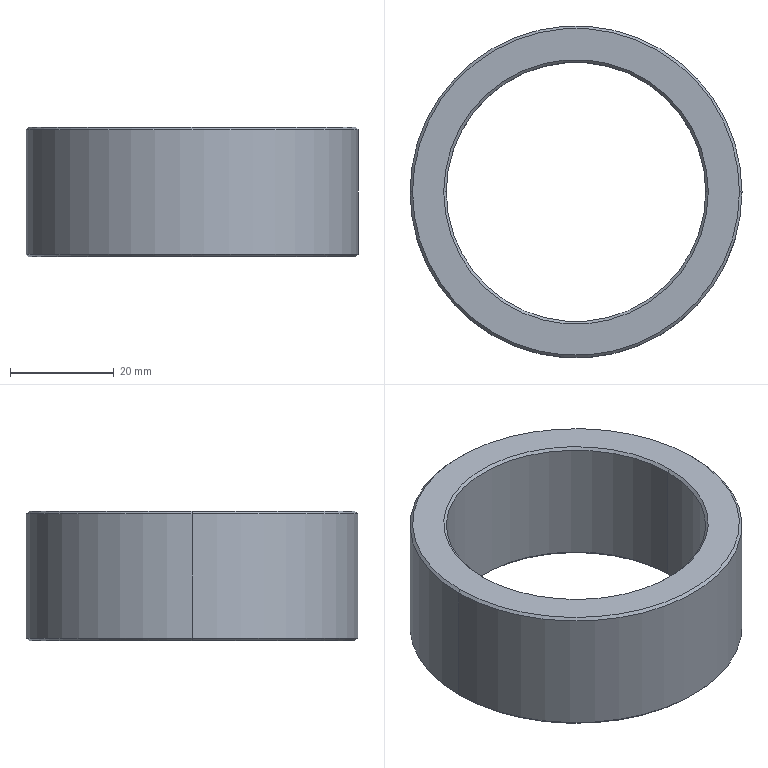Part | SolidWorks | features BaseBody 1 | 1 solid | 14 faces | box 64 x 64 x 25 mm | volume 31248 mm3 | cone 8 | cylinder 4 | plane 2 | commonest cylinder face diameters 50 x2 64 x2
STEP:
#1=CARTESIAN_POINT('',(-25.,0.,0.5));
#2=VERTEX_POINT('',#1);
#3=CARTESIAN_POINT('',(25.,0.,0.5));
#4=VERTEX_POINT('',#3);
#5=CARTESIAN_POINT('',(0.,0.,0.5));
#6=DIRECTION('',(0.,0.,1.));
#7=DIRECTION('',(-1.,0.,0.));
#8=AXIS2_PLACEMENT_3D('',#5,#6,#7);
#9=CIRCLE('',#8,25.);
#10=EDGE_CURVE('',#2,#4,#9,.T.);
#11=ORIENTED_EDGE('',*,*,#10,.T.);
#12=CARTESIAN_POINT('',(25.5,0.,0.));
#13=VERTEX_POINT('',#12);
#14=CARTESIAN_POINT('',(25.25,0.,0.25));
#15=DIRECTION('',(0.7071,0.,-0.7071));
#16=VECTOR('',#15,1000.);
#17=LINE('',#14,#16);
#18=EDGE_CURVE('',#4,#13,#17,.T.);
#19=ORIENTED_EDGE('',*,*,#18,.T.);
#20=CARTESIAN_POINT('',(-25.5,0.,0.));
#21=VERTEX_POINT('',#20);
#22=CARTESIAN_POINT('',(0.,0.,0.));
#23=DIRECTION('',(0.,0.,-1.));
#24=DIRECTION('',(-1.,0.,0.));
#25=AXIS2_PLACEMENT_3D('',#22,#23,#24);
#26=CIRCLE('',#25,25.5);
#27=EDGE_CURVE('',#13,#21,#26,.T.);
#28=ORIENTED_EDGE('',*,*,#27,.T.);
#29=CARTESIAN_POINT('',(-25.25,0.,0.25));
#30=DIRECTION('',(-0.7071,0.,-0.7071));
#31=VECTOR('',#30,1000.);
#32=LINE('',#29,#31);
#33=EDGE_CURVE('',#2,#21,#32,.T.);
#34=ORIENTED_EDGE('',*,*,#33,.F.);
#35=EDGE_LOOP('',(#11,#19,#28,#34));
#36=FACE_OUTER_BOUND('',#35,.T.);
#37=CARTESIAN_POINT('',(0.,0.,0.25));
#38=DIRECTION('',(0.,0.,-1.));
#39=DIRECTION('',(-1.,0.,0.));
#40=AXIS2_PLACEMENT_3D('',#37,#38,#39);
#41=CONICAL_SURFACE('',#40,25.25,0.7854);
#42=ADVANCED_FACE('',(#36),#41,.F.);
#43=CARTESIAN_POINT('',(25.,0.,24.5));
#44=VERTEX_POINT('',#43);
#45=CARTESIAN_POINT('',(-25.,0.,24.5));
#46=VERTEX_POINT('',#45);
#47=CARTESIAN_POINT('',(0.,0.,24.5));
#48=DIRECTION('',(0.,0.,-1.));
#49=DIRECTION('',(-1.,0.,0.));
#50=AXIS2_PLACEMENT_3D('',#47,#48,#49);
#51=CIRCLE('',#50,25.);
#52=EDGE_CURVE('',#44,#46,#51,.T.);
#53=ORIENTED_EDGE('',*,*,#52,.F.);
#54=CARTESIAN_POINT('',(25.,0.,0.));
#55=DIRECTION('',(0.,0.,-1.));
#56=VECTOR('',#55,1000.);
#57=LINE('',#54,#56);
#58=EDGE_CURVE('',#44,#4,#57,.T.);
#59=ORIENTED_EDGE('',*,*,#58,.T.);
#60=ORIENTED_EDGE('',*,*,#10,.F.);
#61=CARTESIAN_POINT('',(-25.,0.,0.));
#62=DIRECTION('',(0.,0.,-1.));
#63=VECTOR('',#62,1000.);
#64=LINE('',#61,#63);
#65=EDGE_CURVE('',#46,#2,#64,.T.);
#66=ORIENTED_EDGE('',*,*,#65,.F.);
#67=EDGE_LOOP('',(#53,#59,#60,#66));
#68=FACE_OUTER_BOUND('',#67,.T.);
#69=CARTESIAN_POINT('',(0.,0.,0.));
#70=DIRECTION('',(0.,0.,-1.));
#71=DIRECTION('',(-1.,0.,0.));
#72=AXIS2_PLACEMENT_3D('',#69,#70,#71);
#73=CYLINDRICAL_SURFACE('',#72,25.);
#74=ADVANCED_FACE('',(#68),#73,.F.);
#75=CARTESIAN_POINT('',(-31.5,0.,0.));
#76=VERTEX_POINT('',#75);
#77=CARTESIAN_POINT('',(31.5,0.,0.));
#78=VERTEX_POINT('',#77);
#79=CARTESIAN_POINT('',(0.,0.,0.));
#80=DIRECTION('',(0.,0.,1.));
#81=DIRECTION('',(-1.,0.,0.));
#82=AXIS2_PLACEMENT_3D('',#79,#80,#81);
#83=CIRCLE('',#82,31.5);
#84=EDGE_CURVE('',#76,#78,#83,.T.);
#85=ORIENTED_EDGE('',*,*,#84,.T.);
#86=CARTESIAN_POINT('',(32.,0.,0.5));
#87=VERTEX_POINT('',#86);
#88=CARTESIAN_POINT('',(31.75,0.,0.25));
#89=DIRECTION('',(0.7071,0.,0.7071));
#90=VECTOR('',#89,1000.);
#91=LINE('',#88,#90);
#92=EDGE_CURVE('',#78,#87,#91,.T.);
#93=ORIENTED_EDGE('',*,*,#92,.T.);
#94=CARTESIAN_POINT('',(-32.,0.,0.5));
#95=VERTEX_POINT('',#94);
#96=CARTESIAN_POINT('',(0.,0.,0.5));
#97=DIRECTION('',(0.,0.,-1.));
#98=DIRECTION('',(-1.,0.,0.));
#99=AXIS2_PLACEMENT_3D('',#96,#97,#98);
#100=CIRCLE('',#99,32.);
#101=EDGE_CURVE('',#87,#95,#100,.T.);
#102=ORIENTED_EDGE('',*,*,#101,.T.);
#103=CARTESIAN_POINT('',(-31.75,0.,0.25));
#104=DIRECTION('',(-0.7071,0.,0.7071));
#105=VECTOR('',#104,1000.);
#106=LINE('',#103,#105);
#107=EDGE_CURVE('',#76,#95,#106,.T.);
#108=ORIENTED_EDGE('',*,*,#107,.F.);
#109=EDGE_LOOP('',(#85,#93,#102,#108));
#110=FACE_OUTER_BOUND('',#109,.T.);
#111=CARTESIAN_POINT('',(0.,0.,0.25));
#112=DIRECTION('',(0.,0.,1.));
#113=DIRECTION('',(-1.,0.,0.));
#114=AXIS2_PLACEMENT_3D('',#111,#112,#113);
#115=CONICAL_SURFACE('',#114,31.75,0.7854);
#116=ADVANCED_FACE('',(#110),#115,.T.);
#117=CARTESIAN_POINT('',(32.,0.,24.5));
#118=VERTEX_POINT('',#117);
#119=CARTESIAN_POINT('',(-32.,0.,24.5));
#120=VERTEX_POINT('',#119);
#121=CARTESIAN_POINT('',(0.,0.,24.5));
#122=DIRECTION('',(0.,0.,1.));
#123=DIRECTION('',(-1.,0.,0.));
#124=AXIS2_PLACEMENT_3D('',#121,#122,#123);
#125=CIRCLE('',#124,32.);
#126=EDGE_CURVE('',#118,#120,#125,.T.);
#127=ORIENTED_EDGE('',*,*,#126,.F.);
#128=CARTESIAN_POINT('',(32.,0.,0.));
#129=DIRECTION('',(0.,0.,-1.));
#130=VECTOR('',#129,1000.);
#131=LINE('',#128,#130);
#132=EDGE_CURVE('',#118,#87,#131,.T.);
#133=ORIENTED_EDGE('',*,*,#132,.T.);
#134=CARTESIAN_POINT('',(0.,0.,0.5));
#135=DIRECTION('',(0.,0.,-1.));
#136=DIRECTION('',(-1.,0.,0.));
#137=AXIS2_PLACEMENT_3D('',#134,#135,#136);
#138=CIRCLE('',#137,32.);
#139=EDGE_CURVE('',#95,#87,#138,.T.);
#140=ORIENTED_EDGE('',*,*,#139,.F.);
#141=CARTESIAN_POINT('',(-32.,0.,0.));
#142=DIRECTION('',(0.,0.,-1.));
#143=VECTOR('',#142,1000.);
#144=LINE('',#141,#143);
#145=EDGE_CURVE('',#120,#95,#144,.T.);
#146=ORIENTED_EDGE('',*,*,#145,.F.);
#147=EDGE_LOOP('',(#127,#133,#140,#146));
#148=FACE_OUTER_BOUND('',#147,.T.);
#149=CARTESIAN_POINT('',(0.,0.,0.));
#150=DIRECTION('',(0.,0.,-1.));
#151=DIRECTION('',(-1.,0.,0.));
#152=AXIS2_PLACEMENT_3D('',#149,#150,#151);
#153=CYLINDRICAL_SURFACE('',#152,32.);
#154=ADVANCED_FACE('',(#148),#153,.T.);
#155=CARTESIAN_POINT('',(-31.5,0.,25.));
#156=VERTEX_POINT('',#155);
#157=CARTESIAN_POINT('',(31.5,0.,25.));
#158=VERTEX_POINT('',#157);
#159=CARTESIAN_POINT('',(0.,0.,25.));
#160=DIRECTION('',(0.,0.,-1.));
#161=DIRECTION('',(-1.,0.,0.));
#162=AXIS2_PLACEMENT_3D('',#159,#160,#161);
#163=CIRCLE('',#162,31.5);
#164=EDGE_CURVE('',#156,#158,#163,.T.);
#165=ORIENTED_EDGE('',*,*,#164,.T.);
#166=CARTESIAN_POINT('',(31.75,0.,24.75));
#167=DIRECTION('',(0.7071,0.,-0.7071));
#168=VECTOR('',#167,1000.);
#169=LINE('',#166,#168);
#170=EDGE_CURVE('',#158,#118,#169,.T.);
#171=ORIENTED_EDGE('',*,*,#170,.T.);
#172=ORIENTED_EDGE('',*,*,#126,.T.);
#173=CARTESIAN_POINT('',(-31.75,0.,24.75));
#174=DIRECTION('',(-0.7071,0.,-0.7071));
#175=VECTOR('',#174,1000.);
#176=LINE('',#173,#175);
#177=EDGE_CURVE('',#156,#120,#176,.T.);
#178=ORIENTED_EDGE('',*,*,#177,.F.);
#179=EDGE_LOOP('',(#165,#171,#172,#178));
#180=FACE_OUTER_BOUND('',#179,.T.);
#181=CARTESIAN_POINT('',(0.,0.,24.75));
#182=DIRECTION('',(0.,0.,-1.));
#183=DIRECTION('',(-1.,0.,0.));
#184=AXIS2_PLACEMENT_3D('',#181,#182,#183);
#185=CONICAL_SURFACE('',#184,31.75,0.7854);
#186=ADVANCED_FACE('',(#180),#185,.T.);
#187=CARTESIAN_POINT('',(0.,0.,24.5));
#188=DIRECTION('',(0.,0.,-1.));
#189=DIRECTION('',(-1.,0.,0.));
#190=AXIS2_PLACEMENT_3D('',#187,#188,#189);
#191=CIRCLE('',#190,25.);
#192=EDGE_CURVE('',#46,#44,#191,.T.);
#193=ORIENTED_EDGE('',*,*,#192,.T.);
#194=CARTESIAN_POINT('',(25.5,0.,25.));
#195=VERTEX_POINT('',#194);
#196=CARTESIAN_POINT('',(25.25,0.,24.75));
#197=DIRECTION('',(0.7071,0.,0.7071));
#198=VECTOR('',#197,1000.);
#199=LINE('',#196,#198);
#200=EDGE_CURVE('',#44,#195,#199,.T.);
#201=ORIENTED_EDGE('',*,*,#200,.T.);
#202=CARTESIAN_POINT('',(-25.5,0.,25.));
#203=VERTEX_POINT('',#202);
#204=CARTESIAN_POINT('',(0.,0.,25.));
#205=DIRECTION('',(0.,0.,1.));
#206=DIRECTION('',(-1.,0.,0.));
#207=AXIS2_PLACEMENT_3D('',#204,#205,#206);
#208=CIRCLE('',#207,25.5);
#209=EDGE_CURVE('',#195,#203,#208,.T.);
#210=ORIENTED_EDGE('',*,*,#209,.T.);
#211=CARTESIAN_POINT('',(-25.25,0.,24.75));
#212=DIRECTION('',(-0.7071,0.,0.7071));
#213=VECTOR('',#212,1000.);
#214=LINE('',#211,#213);
#215=EDGE_CURVE('',#46,#203,#214,.T.);
#216=ORIENTED_EDGE('',*,*,#215,.F.);
#217=EDGE_LOOP('',(#193,#201,#210,#216));
#218=FACE_OUTER_BOUND('',#217,.T.);
#219=CARTESIAN_POINT('',(0.,0.,24.75));
#220=DIRECTION('',(0.,0.,1.));
#221=DIRECTION('',(-1.,0.,0.));
#222=AXIS2_PLACEMENT_3D('',#219,#220,#221);
#223=CONICAL_SURFACE('',#222,25.25,0.7854);
#224=ADVANCED_FACE('',(#218),#223,.F.);
#225=CARTESIAN_POINT('',(0.,0.,0.));
#226=DIRECTION('',(0.,0.,-1.));
#227=DIRECTION('',(-1.,0.,0.));
#228=AXIS2_PLACEMENT_3D('',#225,#226,#227);
#229=CIRCLE('',#228,25.5);
#230=EDGE_CURVE('',#21,#13,#229,.T.);
#231=ORIENTED_EDGE('',*,*,#230,.F.);
#232=ORIENTED_EDGE('',*,*,#27,.F.);
#233=EDGE_LOOP('',(#231,#232));
#234=FACE_BOUND('',#233,.T.);
#235=ORIENTED_EDGE('',*,*,#84,.F.);
#236=CARTESIAN_POINT('',(0.,0.,0.));
#237=DIRECTION('',(0.,0.,1.));
#238=DIRECTION('',(-1.,0.,0.));
#239=AXIS2_PLACEMENT_3D('',#236,#237,#238);
#240=CIRCLE('',#239,31.5);
#241=EDGE_CURVE('',#78,#76,#240,.T.);
#242=ORIENTED_EDGE('',*,*,#241,.F.);
#243=EDGE_LOOP('',(#235,#242));
#244=FACE_OUTER_BOUND('',#243,.T.);
#245=CARTESIAN_POINT('',(0.,0.,0.));
#246=DIRECTION('',(0.,0.,1.));
#247=DIRECTION('',(1.,0.,0.));
#248=AXIS2_PLACEMENT_3D('',#245,#246,#247);
#249=PLANE('',#248);
#250=ADVANCED_FACE('',(#234,#244),#249,.F.);
#251=CARTESIAN_POINT('',(0.,0.,25.));
#252=DIRECTION('',(0.,0.,1.));
#253=DIRECTION('',(-1.,0.,0.));
#254=AXIS2_PLACEMENT_3D('',#251,#252,#253);
#255=CIRCLE('',#254,25.5);
#256=EDGE_CURVE('',#203,#195,#255,.T.);
#257=ORIENTED_EDGE('',*,*,#256,.F.);
#258=ORIENTED_EDGE('',*,*,#209,.F.);
#259=EDGE_LOOP('',(#257,#258));
#260=FACE_BOUND('',#259,.T.);
#261=ORIENTED_EDGE('',*,*,#164,.F.);
#262=CARTESIAN_POINT('',(0.,0.,25.));
#263=DIRECTION('',(0.,0.,-1.));
#264=DIRECTION('',(-1.,0.,0.));
#265=AXIS2_PLACEMENT_3D('',#262,#263,#264);
#266=CIRCLE('',#265,31.5);
#267=EDGE_CURVE('',#158,#156,#266,.T.);
#268=ORIENTED_EDGE('',*,*,#267,.F.);
#269=EDGE_LOOP('',(#261,#268));
#270=FACE_OUTER_BOUND('',#269,.T.);
#271=CARTESIAN_POINT('',(0.,0.,25.));
#272=DIRECTION('',(0.,0.,1.));
#273=DIRECTION('',(1.,0.,0.));
#274=AXIS2_PLACEMENT_3D('',#271,#272,#273);
#275=PLANE('',#274);
#276=ADVANCED_FACE('',(#260,#270),#275,.T.);
#277=ORIENTED_EDGE('',*,*,#200,.F.);
#278=ORIENTED_EDGE('',*,*,#52,.T.);
#279=ORIENTED_EDGE('',*,*,#215,.T.);
#280=ORIENTED_EDGE('',*,*,#256,.T.);
#281=EDGE_LOOP('',(#277,#278,#279,#280));
#282=FACE_OUTER_BOUND('',#281,.T.);
#283=CARTESIAN_POINT('',(0.,0.,24.75));
#284=DIRECTION('',(0.,0.,1.));
#285=DIRECTION('',(-1.,0.,0.));
#286=AXIS2_PLACEMENT_3D('',#283,#284,#285);
#287=CONICAL_SURFACE('',#286,25.25,0.7854);
#288=ADVANCED_FACE('',(#282),#287,.F.);
#289=ORIENTED_EDGE('',*,*,#170,.F.);
#290=ORIENTED_EDGE('',*,*,#267,.T.);
#291=ORIENTED_EDGE('',*,*,#177,.T.);
#292=CARTESIAN_POINT('',(0.,0.,24.5));
#293=DIRECTION('',(0.,0.,1.));
#294=DIRECTION('',(-1.,0.,0.));
#295=AXIS2_PLACEMENT_3D('',#292,#293,#294);
#296=CIRCLE('',#295,32.);
#297=EDGE_CURVE('',#120,#118,#296,.T.);
#298=ORIENTED_EDGE('',*,*,#297,.T.);
#299=EDGE_LOOP('',(#289,#290,#291,#298));
#300=FACE_OUTER_BOUND('',#299,.T.);
#301=CARTESIAN_POINT('',(0.,0.,24.75));
#302=DIRECTION('',(0.,0.,-1.));
#303=DIRECTION('',(-1.,0.,0.));
#304=AXIS2_PLACEMENT_3D('',#301,#302,#303);
#305=CONICAL_SURFACE('',#304,31.75,0.7854);
#306=ADVANCED_FACE('',(#300),#305,.T.);
#307=ORIENTED_EDGE('',*,*,#132,.F.);
#308=ORIENTED_EDGE('',*,*,#297,.F.);
#309=ORIENTED_EDGE('',*,*,#145,.T.);
#310=ORIENTED_EDGE('',*,*,#101,.F.);
#311=EDGE_LOOP('',(#307,#308,#309,#310));
#312=FACE_OUTER_BOUND('',#311,.T.);
#313=CARTESIAN_POINT('',(0.,0.,0.));
#314=DIRECTION('',(0.,0.,-1.));
#315=DIRECTION('',(-1.,0.,0.));
#316=AXIS2_PLACEMENT_3D('',#313,#314,#315);
#317=CYLINDRICAL_SURFACE('',#316,32.);
#318=ADVANCED_FACE('',(#312),#317,.T.);
#319=ORIENTED_EDGE('',*,*,#92,.F.);
#320=ORIENTED_EDGE('',*,*,#241,.T.);
#321=ORIENTED_EDGE('',*,*,#107,.T.);
#322=ORIENTED_EDGE('',*,*,#139,.T.);
#323=EDGE_LOOP('',(#319,#320,#321,#322));
#324=FACE_OUTER_BOUND('',#323,.T.);
#325=CARTESIAN_POINT('',(0.,0.,0.25));
#326=DIRECTION('',(0.,0.,1.));
#327=DIRECTION('',(-1.,0.,0.));
#328=AXIS2_PLACEMENT_3D('',#325,#326,#327);
#329=CONICAL_SURFACE('',#328,31.75,0.7854);
#330=ADVANCED_FACE('',(#324),#329,.T.);
#331=ORIENTED_EDGE('',*,*,#58,.F.);
#332=ORIENTED_EDGE('',*,*,#192,.F.);
#333=ORIENTED_EDGE('',*,*,#65,.T.);
#334=CARTESIAN_POINT('',(0.,0.,0.5));
#335=DIRECTION('',(0.,0.,1.));
#336=DIRECTION('',(-1.,0.,0.));
#337=AXIS2_PLACEMENT_3D('',#334,#335,#336);
#338=CIRCLE('',#337,25.);
#339=EDGE_CURVE('',#4,#2,#338,.T.);
#340=ORIENTED_EDGE('',*,*,#339,.F.);
#341=EDGE_LOOP('',(#331,#332,#333,#340));
#342=FACE_OUTER_BOUND('',#341,.T.);
#343=CARTESIAN_POINT('',(0.,0.,0.));
#344=DIRECTION('',(0.,0.,-1.));
#345=DIRECTION('',(-1.,0.,0.));
#346=AXIS2_PLACEMENT_3D('',#343,#344,#345);
#347=CYLINDRICAL_SURFACE('',#346,25.);
#348=ADVANCED_FACE('',(#342),#347,.F.);
#349=ORIENTED_EDGE('',*,*,#18,.F.);
#350=ORIENTED_EDGE('',*,*,#339,.T.);
#351=ORIENTED_EDGE('',*,*,#33,.T.);
#352=ORIENTED_EDGE('',*,*,#230,.T.);
#353=EDGE_LOOP('',(#349,#350,#351,#352));
#354=FACE_OUTER_BOUND('',#353,.T.);
#355=CARTESIAN_POINT('',(0.,0.,0.25));
#356=DIRECTION('',(0.,0.,-1.));
#357=DIRECTION('',(-1.,0.,0.));
#358=AXIS2_PLACEMENT_3D('',#355,#356,#357);
#359=CONICAL_SURFACE('',#358,25.25,0.7854);
#360=ADVANCED_FACE('',(#354),#359,.F.);
#361=CLOSED_SHELL('',(#42,#74,#116,#154,#186,#224,#250,#276,#288,#306,#318,#330,#348,#360));
#362=MANIFOLD_SOLID_BREP('',#361);
#363=CARTESIAN_POINT('',(0.,0.,0.));
#364=DIRECTION('',(0.,0.,1.));
#365=DIRECTION('',(1.,0.,0.));
#366=AXIS2_PLACEMENT_3D('',#363,#364,#365);
#367=(LENGTH_UNIT()NAMED_UNIT(*)SI_UNIT(.MILLI.,.METRE.));
#368=UNCERTAINTY_MEASURE_WITH_UNIT(LENGTH_MEASURE(0.00001),#367,'','');
#369=(NAMED_UNIT(*)PLANE_ANGLE_UNIT()SI_UNIT($,.RADIAN.));
#370=(NAMED_UNIT(*)SI_UNIT($,.STERADIAN.)SOLID_ANGLE_UNIT());
#371=(GEOMETRIC_REPRESENTATION_CONTEXT(3)GLOBAL_UNCERTAINTY_ASSIGNED_CONTEXT((#368))GLOBAL_UNIT_ASSIGNED_CONTEXT((#367,#369,#370))REPRESENTATION_CONTEXT('',''));
#372=ADVANCED_BREP_SHAPE_REPRESENTATION('',(#362,#366),#371);